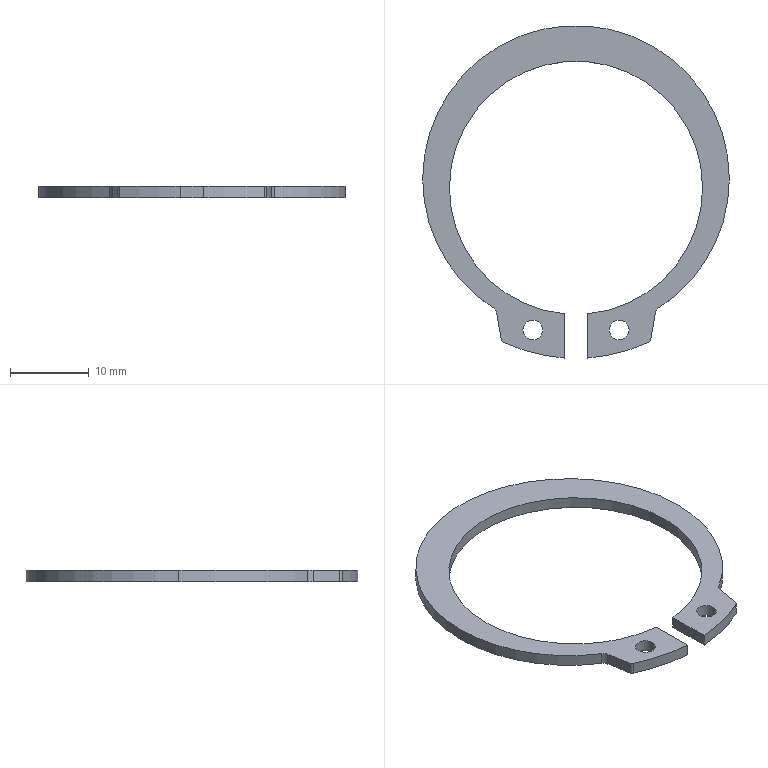Part | SolidWorks | features Extrusion 1 | 1 solid | 22 faces | box 39 x 42.278 x 1.5 mm | volume 631.207 mm3 | cylinder 16 | plane 6 | commonest cylinder face diameters 2.5 x4 32.2 x3 39 x3 1 x2 2 x2 43.4 x2
STEP:
#1=CARTESIAN_POINT('',(4.25,-19.212,0.75));
#2=VERTEX_POINT('',#1);
#3=CARTESIAN_POINT('',(6.75,-19.212,0.75));
#4=VERTEX_POINT('',#3);
#5=CARTESIAN_POINT('',(5.5,-19.212,0.75));
#6=DIRECTION('',(0.,0.,1.));
#7=DIRECTION('',(-1.,0.,0.));
#8=AXIS2_PLACEMENT_3D('',#5,#6,#7);
#9=CIRCLE('',#8,1.25);
#10=EDGE_CURVE('',#2,#4,#9,.T.);
#11=ORIENTED_EDGE('',*,*,#10,.T.);
#12=CARTESIAN_POINT('',(6.75,-19.212,-0.75));
#13=VERTEX_POINT('',#12);
#14=CARTESIAN_POINT('',(6.75,-19.212,0.75));
#15=DIRECTION('',(0.,0.,-1.));
#16=VECTOR('',#15,1000.);
#17=LINE('',#14,#16);
#18=EDGE_CURVE('',#4,#13,#17,.T.);
#19=ORIENTED_EDGE('',*,*,#18,.T.);
#20=CARTESIAN_POINT('',(4.25,-19.212,-0.75));
#21=VERTEX_POINT('',#20);
#22=CARTESIAN_POINT('',(5.5,-19.212,-0.75));
#23=DIRECTION('',(0.,0.,1.));
#24=DIRECTION('',(-1.,0.,0.));
#25=AXIS2_PLACEMENT_3D('',#22,#23,#24);
#26=CIRCLE('',#25,1.25);
#27=EDGE_CURVE('',#21,#13,#26,.T.);
#28=ORIENTED_EDGE('',*,*,#27,.F.);
#29=CARTESIAN_POINT('',(4.25,-19.212,0.75));
#30=DIRECTION('',(0.,0.,-1.));
#31=VECTOR('',#30,1000.);
#32=LINE('',#29,#31);
#33=EDGE_CURVE('',#2,#21,#32,.T.);
#34=ORIENTED_EDGE('',*,*,#33,.F.);
#35=EDGE_LOOP('',(#11,#19,#28,#34));
#36=FACE_OUTER_BOUND('',#35,.T.);
#37=CARTESIAN_POINT('',(5.5,-19.212,0.75));
#38=DIRECTION('',(0.,0.,-1.));
#39=DIRECTION('',(-1.,0.,0.));
#40=AXIS2_PLACEMENT_3D('',#37,#38,#39);
#41=CYLINDRICAL_SURFACE('',#40,1.25);
#42=ADVANCED_FACE('',(#36),#41,.F.);
#43=CARTESIAN_POINT('',(-6.75,-19.212,0.75));
#44=VERTEX_POINT('',#43);
#45=CARTESIAN_POINT('',(-4.25,-19.212,0.75));
#46=VERTEX_POINT('',#45);
#47=CARTESIAN_POINT('',(-5.5,-19.212,0.75));
#48=DIRECTION('',(0.,0.,1.));
#49=DIRECTION('',(1.,0.,0.));
#50=AXIS2_PLACEMENT_3D('',#47,#48,#49);
#51=CIRCLE('',#50,1.25);
#52=EDGE_CURVE('',#44,#46,#51,.T.);
#53=ORIENTED_EDGE('',*,*,#52,.T.);
#54=CARTESIAN_POINT('',(-4.25,-19.212,-0.75));
#55=VERTEX_POINT('',#54);
#56=CARTESIAN_POINT('',(-4.25,-19.212,0.75));
#57=DIRECTION('',(0.,0.,-1.));
#58=VECTOR('',#57,1000.);
#59=LINE('',#56,#58);
#60=EDGE_CURVE('',#46,#55,#59,.T.);
#61=ORIENTED_EDGE('',*,*,#60,.T.);
#62=CARTESIAN_POINT('',(-6.75,-19.212,-0.75));
#63=VERTEX_POINT('',#62);
#64=CARTESIAN_POINT('',(-5.5,-19.212,-0.75));
#65=DIRECTION('',(0.,0.,1.));
#66=DIRECTION('',(1.,0.,0.));
#67=AXIS2_PLACEMENT_3D('',#64,#65,#66);
#68=CIRCLE('',#67,1.25);
#69=EDGE_CURVE('',#63,#55,#68,.T.);
#70=ORIENTED_EDGE('',*,*,#69,.F.);
#71=CARTESIAN_POINT('',(-6.75,-19.212,0.75));
#72=DIRECTION('',(0.,0.,-1.));
#73=VECTOR('',#72,1000.);
#74=LINE('',#71,#73);
#75=EDGE_CURVE('',#44,#63,#74,.T.);
#76=ORIENTED_EDGE('',*,*,#75,.F.);
#77=EDGE_LOOP('',(#53,#61,#70,#76));
#78=FACE_OUTER_BOUND('',#77,.T.);
#79=CARTESIAN_POINT('',(-5.5,-19.212,0.75));
#80=DIRECTION('',(0.,0.,-1.));
#81=DIRECTION('',(-1.,0.,0.));
#82=AXIS2_PLACEMENT_3D('',#79,#80,#81);
#83=CYLINDRICAL_SURFACE('',#82,1.25);
#84=ADVANCED_FACE('',(#78),#83,.F.);
#85=CARTESIAN_POINT('',(19.5,0.,0.75));
#86=VERTEX_POINT('',#85);
#87=CARTESIAN_POINT('',(-19.5,0.,0.75));
#88=VERTEX_POINT('',#87);
#89=CARTESIAN_POINT('',(0.,0.,0.75));
#90=DIRECTION('',(0.,0.,1.));
#91=DIRECTION('',(1.,0.,0.));
#92=AXIS2_PLACEMENT_3D('',#89,#90,#91);
#93=CIRCLE('',#92,19.5);
#94=EDGE_CURVE('',#86,#88,#93,.T.);
#95=ORIENTED_EDGE('',*,*,#94,.F.);
#96=CARTESIAN_POINT('',(19.5,0.,-0.75));
#97=VERTEX_POINT('',#96);
#98=CARTESIAN_POINT('',(19.5,0.,0.75));
#99=DIRECTION('',(0.,0.,-1.));
#100=VECTOR('',#99,1000.);
#101=LINE('',#98,#100);
#102=EDGE_CURVE('',#86,#97,#101,.T.);
#103=ORIENTED_EDGE('',*,*,#102,.T.);
#104=CARTESIAN_POINT('',(-19.5,0.,-0.75));
#105=VERTEX_POINT('',#104);
#106=CARTESIAN_POINT('',(0.,0.,-0.75));
#107=DIRECTION('',(0.,0.,1.));
#108=DIRECTION('',(1.,0.,0.));
#109=AXIS2_PLACEMENT_3D('',#106,#107,#108);
#110=CIRCLE('',#109,19.5);
#111=EDGE_CURVE('',#97,#105,#110,.T.);
#112=ORIENTED_EDGE('',*,*,#111,.T.);
#113=CARTESIAN_POINT('',(-19.5,0.,0.75));
#114=DIRECTION('',(0.,0.,-1.));
#115=VECTOR('',#114,1000.);
#116=LINE('',#113,#115);
#117=EDGE_CURVE('',#88,#105,#116,.T.);
#118=ORIENTED_EDGE('',*,*,#117,.F.);
#119=EDGE_LOOP('',(#95,#103,#112,#118));
#120=FACE_OUTER_BOUND('',#119,.T.);
#121=CARTESIAN_POINT('',(0.,0.,0.75));
#122=DIRECTION('',(0.,0.,-1.));
#123=DIRECTION('',(-1.,0.,0.));
#124=AXIS2_PLACEMENT_3D('',#121,#122,#123);
#125=CYLINDRICAL_SURFACE('',#124,19.5);
#126=ADVANCED_FACE('',(#120),#125,.T.);
#127=CARTESIAN_POINT('',(-10.532,-16.411,0.75));
#128=VERTEX_POINT('',#127);
#129=CARTESIAN_POINT('',(0.,0.,0.75));
#130=DIRECTION('',(0.,0.,1.));
#131=DIRECTION('',(1.,0.,0.));
#132=AXIS2_PLACEMENT_3D('',#129,#130,#131);
#133=CIRCLE('',#132,19.5);
#134=EDGE_CURVE('',#88,#128,#133,.T.);
#135=ORIENTED_EDGE('',*,*,#134,.F.);
#136=ORIENTED_EDGE('',*,*,#117,.T.);
#137=CARTESIAN_POINT('',(-10.532,-16.411,-0.75));
#138=VERTEX_POINT('',#137);
#139=CARTESIAN_POINT('',(0.,0.,-0.75));
#140=DIRECTION('',(0.,0.,1.));
#141=DIRECTION('',(1.,0.,0.));
#142=AXIS2_PLACEMENT_3D('',#139,#140,#141);
#143=CIRCLE('',#142,19.5);
#144=EDGE_CURVE('',#105,#138,#143,.T.);
#145=ORIENTED_EDGE('',*,*,#144,.T.);
#146=CARTESIAN_POINT('',(-10.532,-16.411,0.75));
#147=DIRECTION('',(0.,0.,-1.));
#148=VECTOR('',#147,1000.);
#149=LINE('',#146,#148);
#150=EDGE_CURVE('',#128,#138,#149,.T.);
#151=ORIENTED_EDGE('',*,*,#150,.F.);
#152=EDGE_LOOP('',(#135,#136,#145,#151));
#153=FACE_OUTER_BOUND('',#152,.T.);
#154=CARTESIAN_POINT('',(0.,0.,0.75));
#155=DIRECTION('',(0.,0.,-1.));
#156=DIRECTION('',(-1.,0.,0.));
#157=AXIS2_PLACEMENT_3D('',#154,#155,#156);
#158=CYLINDRICAL_SURFACE('',#157,19.5);
#159=ADVANCED_FACE('',(#153),#158,.T.);
#160=CARTESIAN_POINT('',(16.1,-1.13,0.75));
#161=VERTEX_POINT('',#160);
#162=CARTESIAN_POINT('',(1.5,-17.16,0.75));
#163=VERTEX_POINT('',#162);
#164=CARTESIAN_POINT('',(0.,-1.13,0.75));
#165=DIRECTION('',(0.,0.,-1.));
#166=DIRECTION('',(1.,0.,0.));
#167=AXIS2_PLACEMENT_3D('',#164,#165,#166);
#168=CIRCLE('',#167,16.1);
#169=EDGE_CURVE('',#161,#163,#168,.T.);
#170=ORIENTED_EDGE('',*,*,#169,.F.);
#171=CARTESIAN_POINT('',(16.1,-1.13,-0.75));
#172=VERTEX_POINT('',#171);
#173=CARTESIAN_POINT('',(16.1,-1.13,0.75));
#174=DIRECTION('',(0.,0.,-1.));
#175=VECTOR('',#174,1000.);
#176=LINE('',#173,#175);
#177=EDGE_CURVE('',#161,#172,#176,.T.);
#178=ORIENTED_EDGE('',*,*,#177,.T.);
#179=CARTESIAN_POINT('',(1.5,-17.16,-0.75));
#180=VERTEX_POINT('',#179);
#181=CARTESIAN_POINT('',(0.,-1.13,-0.75));
#182=DIRECTION('',(0.,0.,-1.));
#183=DIRECTION('',(1.,0.,0.));
#184=AXIS2_PLACEMENT_3D('',#181,#182,#183);
#185=CIRCLE('',#184,16.1);
#186=EDGE_CURVE('',#172,#180,#185,.T.);
#187=ORIENTED_EDGE('',*,*,#186,.T.);
#188=CARTESIAN_POINT('',(1.5,-17.16,0.75));
#189=DIRECTION('',(0.,0.,-1.));
#190=VECTOR('',#189,1000.);
#191=LINE('',#188,#190);
#192=EDGE_CURVE('',#163,#180,#191,.T.);
#193=ORIENTED_EDGE('',*,*,#192,.F.);
#194=EDGE_LOOP('',(#170,#178,#187,#193));
#195=FACE_OUTER_BOUND('',#194,.T.);
#196=CARTESIAN_POINT('',(0.,-1.13,0.75));
#197=DIRECTION('',(0.,0.,-1.));
#198=DIRECTION('',(-1.,0.,0.));
#199=AXIS2_PLACEMENT_3D('',#196,#197,#198);
#200=CYLINDRICAL_SURFACE('',#199,16.1);
#201=ADVANCED_FACE('',(#195),#200,.F.);
#202=ORIENTED_EDGE('',*,*,#177,.F.);
#203=CARTESIAN_POINT('',(-16.1,-1.13,0.75));
#204=VERTEX_POINT('',#203);
#205=CARTESIAN_POINT('',(0.,-1.13,0.75));
#206=DIRECTION('',(0.,0.,-1.));
#207=DIRECTION('',(1.,0.,0.));
#208=AXIS2_PLACEMENT_3D('',#205,#206,#207);
#209=CIRCLE('',#208,16.1);
#210=EDGE_CURVE('',#204,#161,#209,.T.);
#211=ORIENTED_EDGE('',*,*,#210,.F.);
#212=CARTESIAN_POINT('',(-16.1,-1.13,-0.75));
#213=VERTEX_POINT('',#212);
#214=CARTESIAN_POINT('',(-16.1,-1.13,0.75));
#215=DIRECTION('',(0.,0.,-1.));
#216=VECTOR('',#215,1000.);
#217=LINE('',#214,#216);
#218=EDGE_CURVE('',#204,#213,#217,.T.);
#219=ORIENTED_EDGE('',*,*,#218,.T.);
#220=CARTESIAN_POINT('',(0.,-1.13,-0.75));
#221=DIRECTION('',(0.,0.,-1.));
#222=DIRECTION('',(1.,0.,0.));
#223=AXIS2_PLACEMENT_3D('',#220,#221,#222);
#224=CIRCLE('',#223,16.1);
#225=EDGE_CURVE('',#213,#172,#224,.T.);
#226=ORIENTED_EDGE('',*,*,#225,.T.);
#227=EDGE_LOOP('',(#202,#211,#219,#226));
#228=FACE_OUTER_BOUND('',#227,.T.);
#229=CARTESIAN_POINT('',(0.,-1.13,0.75));
#230=DIRECTION('',(0.,0.,-1.));
#231=DIRECTION('',(-1.,0.,0.));
#232=AXIS2_PLACEMENT_3D('',#229,#230,#231);
#233=CYLINDRICAL_SURFACE('',#232,16.1);
#234=ADVANCED_FACE('',(#228),#233,.F.);
#235=ORIENTED_EDGE('',*,*,#52,.F.);
#236=CARTESIAN_POINT('',(-5.5,-19.212,0.75));
#237=DIRECTION('',(0.,0.,1.));
#238=DIRECTION('',(1.,0.,0.));
#239=AXIS2_PLACEMENT_3D('',#236,#237,#238);
#240=CIRCLE('',#239,1.25);
#241=EDGE_CURVE('',#46,#44,#240,.T.);
#242=ORIENTED_EDGE('',*,*,#241,.F.);
#243=EDGE_LOOP('',(#235,#242));
#244=FACE_BOUND('',#243,.T.);
#245=CARTESIAN_POINT('',(-10.087,-17.079,0.75));
#246=VERTEX_POINT('',#245);
#247=CARTESIAN_POINT('',(-11.072,-17.253,0.75));
#248=DIRECTION('',(0.,0.,-1.));
#249=DIRECTION('',(1.,0.,0.));
#250=AXIS2_PLACEMENT_3D('',#247,#248,#249);
#251=CIRCLE('',#250,1.);
#252=EDGE_CURVE('',#128,#246,#251,.T.);
#253=ORIENTED_EDGE('',*,*,#252,.T.);
#254=CARTESIAN_POINT('',(-9.5,-20.408,0.75));
#255=VERTEX_POINT('',#254);
#256=CARTESIAN_POINT('',(-10.087,-17.079,0.75));
#257=DIRECTION('',(0.1736,-0.9848,0.));
#258=VECTOR('',#257,1000.);
#259=LINE('',#256,#258);
#260=EDGE_CURVE('',#246,#255,#259,.T.);
#261=ORIENTED_EDGE('',*,*,#260,.T.);
#262=CARTESIAN_POINT('',(-9.22,-20.774,0.75));
#263=VERTEX_POINT('',#262);
#264=CARTESIAN_POINT('',(-9.008,-20.321,0.75));
#265=DIRECTION('',(0.,0.,1.));
#266=DIRECTION('',(-1.,0.,0.));
#267=AXIS2_PLACEMENT_3D('',#264,#265,#266);
#268=CIRCLE('',#267,0.5);
#269=EDGE_CURVE('',#255,#263,#268,.T.);
#270=ORIENTED_EDGE('',*,*,#269,.T.);
#271=CARTESIAN_POINT('',(-1.5,-22.778,0.75));
#272=VERTEX_POINT('',#271);
#273=CARTESIAN_POINT('',(0.,-1.13,0.75));
#274=DIRECTION('',(0.,0.,1.));
#275=DIRECTION('',(-1.,0.,0.));
#276=AXIS2_PLACEMENT_3D('',#273,#274,#275);
#277=CIRCLE('',#276,21.7);
#278=EDGE_CURVE('',#263,#272,#277,.T.);
#279=ORIENTED_EDGE('',*,*,#278,.T.);
#280=CARTESIAN_POINT('',(-1.5,-17.16,0.75));
#281=VERTEX_POINT('',#280);
#282=CARTESIAN_POINT('',(-1.5,-17.16,0.75));
#283=DIRECTION('',(0.,1.,0.));
#284=VECTOR('',#283,1000.);
#285=LINE('',#282,#284);
#286=EDGE_CURVE('',#272,#281,#285,.T.);
#287=ORIENTED_EDGE('',*,*,#286,.T.);
#288=CARTESIAN_POINT('',(0.,-1.13,0.75));
#289=DIRECTION('',(0.,0.,-1.));
#290=DIRECTION('',(1.,0.,0.));
#291=AXIS2_PLACEMENT_3D('',#288,#289,#290);
#292=CIRCLE('',#291,16.1);
#293=EDGE_CURVE('',#281,#204,#292,.T.);
#294=ORIENTED_EDGE('',*,*,#293,.T.);
#295=ORIENTED_EDGE('',*,*,#210,.T.);
#296=ORIENTED_EDGE('',*,*,#169,.T.);
#297=CARTESIAN_POINT('',(1.5,-22.778,0.75));
#298=VERTEX_POINT('',#297);
#299=CARTESIAN_POINT('',(1.5,-17.16,0.75));
#300=DIRECTION('',(0.,-1.,0.));
#301=VECTOR('',#300,1000.);
#302=LINE('',#299,#301);
#303=EDGE_CURVE('',#163,#298,#302,.T.);
#304=ORIENTED_EDGE('',*,*,#303,.T.);
#305=CARTESIAN_POINT('',(9.22,-20.774,0.75));
#306=VERTEX_POINT('',#305);
#307=CARTESIAN_POINT('',(0.,-1.13,0.75));
#308=DIRECTION('',(0.,0.,1.));
#309=DIRECTION('',(1.,0.,0.));
#310=AXIS2_PLACEMENT_3D('',#307,#308,#309);
#311=CIRCLE('',#310,21.7);
#312=EDGE_CURVE('',#298,#306,#311,.T.);
#313=ORIENTED_EDGE('',*,*,#312,.T.);
#314=CARTESIAN_POINT('',(9.5,-20.408,0.75));
#315=VERTEX_POINT('',#314);
#316=CARTESIAN_POINT('',(9.008,-20.321,0.75));
#317=DIRECTION('',(0.,0.,1.));
#318=DIRECTION('',(1.,0.,0.));
#319=AXIS2_PLACEMENT_3D('',#316,#317,#318);
#320=CIRCLE('',#319,0.5);
#321=EDGE_CURVE('',#306,#315,#320,.T.);
#322=ORIENTED_EDGE('',*,*,#321,.T.);
#323=CARTESIAN_POINT('',(10.087,-17.079,0.75));
#324=VERTEX_POINT('',#323);
#325=CARTESIAN_POINT('',(10.087,-17.079,0.75));
#326=DIRECTION('',(0.1736,0.9848,0.));
#327=VECTOR('',#326,1000.);
#328=LINE('',#325,#327);
#329=EDGE_CURVE('',#315,#324,#328,.T.);
#330=ORIENTED_EDGE('',*,*,#329,.T.);
#331=CARTESIAN_POINT('',(10.532,-16.411,0.75));
#332=VERTEX_POINT('',#331);
#333=CARTESIAN_POINT('',(11.072,-17.253,0.75));
#334=DIRECTION('',(0.,0.,-1.));
#335=DIRECTION('',(-1.,0.,0.));
#336=AXIS2_PLACEMENT_3D('',#333,#334,#335);
#337=CIRCLE('',#336,1.);
#338=EDGE_CURVE('',#324,#332,#337,.T.);
#339=ORIENTED_EDGE('',*,*,#338,.T.);
#340=CARTESIAN_POINT('',(0.,0.,0.75));
#341=DIRECTION('',(0.,0.,1.));
#342=DIRECTION('',(1.,0.,0.));
#343=AXIS2_PLACEMENT_3D('',#340,#341,#342);
#344=CIRCLE('',#343,19.5);
#345=EDGE_CURVE('',#332,#86,#344,.T.);
#346=ORIENTED_EDGE('',*,*,#345,.T.);
#347=ORIENTED_EDGE('',*,*,#94,.T.);
#348=ORIENTED_EDGE('',*,*,#134,.T.);
#349=EDGE_LOOP('',(#253,#261,#270,#279,#287,#294,#295,#296,#304,#313,#322,#330,#339,#346,#347,#348));
#350=FACE_OUTER_BOUND('',#349,.T.);
#351=ORIENTED_EDGE('',*,*,#10,.F.);
#352=CARTESIAN_POINT('',(5.5,-19.212,0.75));
#353=DIRECTION('',(0.,0.,1.));
#354=DIRECTION('',(-1.,0.,0.));
#355=AXIS2_PLACEMENT_3D('',#352,#353,#354);
#356=CIRCLE('',#355,1.25);
#357=EDGE_CURVE('',#4,#2,#356,.T.);
#358=ORIENTED_EDGE('',*,*,#357,.F.);
#359=EDGE_LOOP('',(#351,#358));
#360=FACE_BOUND('',#359,.T.);
#361=CARTESIAN_POINT('',(-11.072,-17.253,0.75));
#362=DIRECTION('',(0.,0.,1.));
#363=DIRECTION('',(1.,0.,0.));
#364=AXIS2_PLACEMENT_3D('',#361,#362,#363);
#365=PLANE('',#364);
#366=ADVANCED_FACE('',(#244,#350,#360),#365,.T.);
#367=ORIENTED_EDGE('',*,*,#150,.T.);
#368=CARTESIAN_POINT('',(-10.087,-17.079,-0.75));
#369=VERTEX_POINT('',#368);
#370=CARTESIAN_POINT('',(-11.072,-17.253,-0.75));
#371=DIRECTION('',(0.,0.,-1.));
#372=DIRECTION('',(1.,0.,0.));
#373=AXIS2_PLACEMENT_3D('',#370,#371,#372);
#374=CIRCLE('',#373,1.);
#375=EDGE_CURVE('',#138,#369,#374,.T.);
#376=ORIENTED_EDGE('',*,*,#375,.T.);
#377=CARTESIAN_POINT('',(-10.087,-17.079,0.75));
#378=DIRECTION('',(0.,0.,-1.));
#379=VECTOR('',#378,1000.);
#380=LINE('',#377,#379);
#381=EDGE_CURVE('',#246,#369,#380,.T.);
#382=ORIENTED_EDGE('',*,*,#381,.F.);
#383=ORIENTED_EDGE('',*,*,#252,.F.);
#384=EDGE_LOOP('',(#367,#376,#382,#383));
#385=FACE_OUTER_BOUND('',#384,.T.);
#386=CARTESIAN_POINT('',(-11.072,-17.253,0.75));
#387=DIRECTION('',(0.,0.,-1.));
#388=DIRECTION('',(-1.,0.,0.));
#389=AXIS2_PLACEMENT_3D('',#386,#387,#388);
#390=CYLINDRICAL_SURFACE('',#389,1.);
#391=ADVANCED_FACE('',(#385),#390,.F.);
#392=ORIENTED_EDGE('',*,*,#381,.T.);
#393=CARTESIAN_POINT('',(-9.5,-20.408,-0.75));
#394=VERTEX_POINT('',#393);
#395=CARTESIAN_POINT('',(-10.087,-17.079,-0.75));
#396=DIRECTION('',(0.1736,-0.9848,0.));
#397=VECTOR('',#396,1000.);
#398=LINE('',#395,#397);
#399=EDGE_CURVE('',#369,#394,#398,.T.);
#400=ORIENTED_EDGE('',*,*,#399,.T.);
#401=CARTESIAN_POINT('',(-9.5,-20.408,0.75));
#402=DIRECTION('',(0.,0.,-1.));
#403=VECTOR('',#402,1000.);
#404=LINE('',#401,#403);
#405=EDGE_CURVE('',#255,#394,#404,.T.);
#406=ORIENTED_EDGE('',*,*,#405,.F.);
#407=ORIENTED_EDGE('',*,*,#260,.F.);
#408=EDGE_LOOP('',(#392,#400,#406,#407));
#409=FACE_OUTER_BOUND('',#408,.T.);
#410=CARTESIAN_POINT('',(-10.087,-17.079,0.75));
#411=DIRECTION('',(0.9848,0.1736,0.));
#412=DIRECTION('',(-0.1736,0.9848,0.));
#413=AXIS2_PLACEMENT_3D('',#410,#411,#412);
#414=PLANE('',#413);
#415=ADVANCED_FACE('',(#409),#414,.F.);
#416=ORIENTED_EDGE('',*,*,#405,.T.);
#417=CARTESIAN_POINT('',(-9.22,-20.774,-0.75));
#418=VERTEX_POINT('',#417);
#419=CARTESIAN_POINT('',(-9.008,-20.321,-0.75));
#420=DIRECTION('',(0.,0.,1.));
#421=DIRECTION('',(-1.,0.,0.));
#422=AXIS2_PLACEMENT_3D('',#419,#420,#421);
#423=CIRCLE('',#422,0.5);
#424=EDGE_CURVE('',#394,#418,#423,.T.);
#425=ORIENTED_EDGE('',*,*,#424,.T.);
#426=CARTESIAN_POINT('',(-9.22,-20.774,0.75));
#427=DIRECTION('',(0.,0.,-1.));
#428=VECTOR('',#427,1000.);
#429=LINE('',#426,#428);
#430=EDGE_CURVE('',#263,#418,#429,.T.);
#431=ORIENTED_EDGE('',*,*,#430,.F.);
#432=ORIENTED_EDGE('',*,*,#269,.F.);
#433=EDGE_LOOP('',(#416,#425,#431,#432));
#434=FACE_OUTER_BOUND('',#433,.T.);
#435=CARTESIAN_POINT('',(-9.008,-20.321,0.75));
#436=DIRECTION('',(0.,0.,-1.));
#437=DIRECTION('',(-1.,0.,0.));
#438=AXIS2_PLACEMENT_3D('',#435,#436,#437);
#439=CYLINDRICAL_SURFACE('',#438,0.5);
#440=ADVANCED_FACE('',(#434),#439,.T.);
#441=ORIENTED_EDGE('',*,*,#430,.T.);
#442=CARTESIAN_POINT('',(-1.5,-22.778,-0.75));
#443=VERTEX_POINT('',#442);
#444=CARTESIAN_POINT('',(0.,-1.13,-0.75));
#445=DIRECTION('',(0.,0.,1.));
#446=DIRECTION('',(-1.,0.,0.));
#447=AXIS2_PLACEMENT_3D('',#444,#445,#446);
#448=CIRCLE('',#447,21.7);
#449=EDGE_CURVE('',#418,#443,#448,.T.);
#450=ORIENTED_EDGE('',*,*,#449,.T.);
#451=CARTESIAN_POINT('',(-1.5,-22.778,0.75));
#452=DIRECTION('',(0.,0.,-1.));
#453=VECTOR('',#452,1000.);
#454=LINE('',#451,#453);
#455=EDGE_CURVE('',#272,#443,#454,.T.);
#456=ORIENTED_EDGE('',*,*,#455,.F.);
#457=ORIENTED_EDGE('',*,*,#278,.F.);
#458=EDGE_LOOP('',(#441,#450,#456,#457));
#459=FACE_OUTER_BOUND('',#458,.T.);
#460=CARTESIAN_POINT('',(0.,-1.13,0.75));
#461=DIRECTION('',(0.,0.,-1.));
#462=DIRECTION('',(-1.,0.,0.));
#463=AXIS2_PLACEMENT_3D('',#460,#461,#462);
#464=CYLINDRICAL_SURFACE('',#463,21.7);
#465=ADVANCED_FACE('',(#459),#464,.T.);
#466=ORIENTED_EDGE('',*,*,#455,.T.);
#467=CARTESIAN_POINT('',(-1.5,-17.16,-0.75));
#468=VERTEX_POINT('',#467);
#469=CARTESIAN_POINT('',(-1.5,-17.16,-0.75));
#470=DIRECTION('',(0.,1.,0.));
#471=VECTOR('',#470,1000.);
#472=LINE('',#469,#471);
#473=EDGE_CURVE('',#443,#468,#472,.T.);
#474=ORIENTED_EDGE('',*,*,#473,.T.);
#475=CARTESIAN_POINT('',(-1.5,-17.16,0.75));
#476=DIRECTION('',(0.,0.,-1.));
#477=VECTOR('',#476,1000.);
#478=LINE('',#475,#477);
#479=EDGE_CURVE('',#281,#468,#478,.T.);
#480=ORIENTED_EDGE('',*,*,#479,.F.);
#481=ORIENTED_EDGE('',*,*,#286,.F.);
#482=EDGE_LOOP('',(#466,#474,#480,#481));
#483=FACE_OUTER_BOUND('',#482,.T.);
#484=CARTESIAN_POINT('',(-1.5,-17.16,0.75));
#485=DIRECTION('',(-1.,0.,0.));
#486=DIRECTION('',(0.,-1.,0.));
#487=AXIS2_PLACEMENT_3D('',#484,#485,#486);
#488=PLANE('',#487);
#489=ADVANCED_FACE('',(#483),#488,.F.);
#490=ORIENTED_EDGE('',*,*,#218,.F.);
#491=ORIENTED_EDGE('',*,*,#293,.F.);
#492=ORIENTED_EDGE('',*,*,#479,.T.);
#493=CARTESIAN_POINT('',(0.,-1.13,-0.75));
#494=DIRECTION('',(0.,0.,-1.));
#495=DIRECTION('',(1.,0.,0.));
#496=AXIS2_PLACEMENT_3D('',#493,#494,#495);
#497=CIRCLE('',#496,16.1);
#498=EDGE_CURVE('',#468,#213,#497,.T.);
#499=ORIENTED_EDGE('',*,*,#498,.T.);
#500=EDGE_LOOP('',(#490,#491,#492,#499));
#501=FACE_OUTER_BOUND('',#500,.T.);
#502=CARTESIAN_POINT('',(0.,-1.13,0.75));
#503=DIRECTION('',(0.,0.,-1.));
#504=DIRECTION('',(-1.,0.,0.));
#505=AXIS2_PLACEMENT_3D('',#502,#503,#504);
#506=CYLINDRICAL_SURFACE('',#505,16.1);
#507=ADVANCED_FACE('',(#501),#506,.F.);
#508=ORIENTED_EDGE('',*,*,#192,.T.);
#509=CARTESIAN_POINT('',(1.5,-22.778,-0.75));
#510=VERTEX_POINT('',#509);
#511=CARTESIAN_POINT('',(1.5,-17.16,-0.75));
#512=DIRECTION('',(0.,-1.,0.));
#513=VECTOR('',#512,1000.);
#514=LINE('',#511,#513);
#515=EDGE_CURVE('',#180,#510,#514,.T.);
#516=ORIENTED_EDGE('',*,*,#515,.T.);
#517=CARTESIAN_POINT('',(1.5,-22.778,0.75));
#518=DIRECTION('',(0.,0.,-1.));
#519=VECTOR('',#518,1000.);
#520=LINE('',#517,#519);
#521=EDGE_CURVE('',#298,#510,#520,.T.);
#522=ORIENTED_EDGE('',*,*,#521,.F.);
#523=ORIENTED_EDGE('',*,*,#303,.F.);
#524=EDGE_LOOP('',(#508,#516,#522,#523));
#525=FACE_OUTER_BOUND('',#524,.T.);
#526=CARTESIAN_POINT('',(1.5,-17.16,0.75));
#527=DIRECTION('',(1.,0.,0.));
#528=DIRECTION('',(0.,1.,0.));
#529=AXIS2_PLACEMENT_3D('',#526,#527,#528);
#530=PLANE('',#529);
#531=ADVANCED_FACE('',(#525),#530,.F.);
#532=ORIENTED_EDGE('',*,*,#521,.T.);
#533=CARTESIAN_POINT('',(9.22,-20.774,-0.75));
#534=VERTEX_POINT('',#533);
#535=CARTESIAN_POINT('',(0.,-1.13,-0.75));
#536=DIRECTION('',(0.,0.,1.));
#537=DIRECTION('',(1.,0.,0.));
#538=AXIS2_PLACEMENT_3D('',#535,#536,#537);
#539=CIRCLE('',#538,21.7);
#540=EDGE_CURVE('',#510,#534,#539,.T.);
#541=ORIENTED_EDGE('',*,*,#540,.T.);
#542=CARTESIAN_POINT('',(9.22,-20.774,0.75));
#543=DIRECTION('',(0.,0.,-1.));
#544=VECTOR('',#543,1000.);
#545=LINE('',#542,#544);
#546=EDGE_CURVE('',#306,#534,#545,.T.);
#547=ORIENTED_EDGE('',*,*,#546,.F.);
#548=ORIENTED_EDGE('',*,*,#312,.F.);
#549=EDGE_LOOP('',(#532,#541,#547,#548));
#550=FACE_OUTER_BOUND('',#549,.T.);
#551=CARTESIAN_POINT('',(0.,-1.13,0.75));
#552=DIRECTION('',(0.,0.,-1.));
#553=DIRECTION('',(-1.,0.,0.));
#554=AXIS2_PLACEMENT_3D('',#551,#552,#553);
#555=CYLINDRICAL_SURFACE('',#554,21.7);
#556=ADVANCED_FACE('',(#550),#555,.T.);
#557=ORIENTED_EDGE('',*,*,#546,.T.);
#558=CARTESIAN_POINT('',(9.5,-20.408,-0.75));
#559=VERTEX_POINT('',#558);
#560=CARTESIAN_POINT('',(9.008,-20.321,-0.75));
#561=DIRECTION('',(0.,0.,1.));
#562=DIRECTION('',(1.,0.,0.));
#563=AXIS2_PLACEMENT_3D('',#560,#561,#562);
#564=CIRCLE('',#563,0.5);
#565=EDGE_CURVE('',#534,#559,#564,.T.);
#566=ORIENTED_EDGE('',*,*,#565,.T.);
#567=CARTESIAN_POINT('',(9.5,-20.408,0.75));
#568=DIRECTION('',(0.,0.,-1.));
#569=VECTOR('',#568,1000.);
#570=LINE('',#567,#569);
#571=EDGE_CURVE('',#315,#559,#570,.T.);
#572=ORIENTED_EDGE('',*,*,#571,.F.);
#573=ORIENTED_EDGE('',*,*,#321,.F.);
#574=EDGE_LOOP('',(#557,#566,#572,#573));
#575=FACE_OUTER_BOUND('',#574,.T.);
#576=CARTESIAN_POINT('',(9.008,-20.321,0.75));
#577=DIRECTION('',(0.,0.,-1.));
#578=DIRECTION('',(-1.,0.,0.));
#579=AXIS2_PLACEMENT_3D('',#576,#577,#578);
#580=CYLINDRICAL_SURFACE('',#579,0.5);
#581=ADVANCED_FACE('',(#575),#580,.T.);
#582=ORIENTED_EDGE('',*,*,#571,.T.);
#583=CARTESIAN_POINT('',(10.087,-17.079,-0.75));
#584=VERTEX_POINT('',#583);
#585=CARTESIAN_POINT('',(10.087,-17.079,-0.75));
#586=DIRECTION('',(0.1736,0.9848,0.));
#587=VECTOR('',#586,1000.);
#588=LINE('',#585,#587);
#589=EDGE_CURVE('',#559,#584,#588,.T.);
#590=ORIENTED_EDGE('',*,*,#589,.T.);
#591=CARTESIAN_POINT('',(10.087,-17.079,0.75));
#592=DIRECTION('',(0.,0.,-1.));
#593=VECTOR('',#592,1000.);
#594=LINE('',#591,#593);
#595=EDGE_CURVE('',#324,#584,#594,.T.);
#596=ORIENTED_EDGE('',*,*,#595,.F.);
#597=ORIENTED_EDGE('',*,*,#329,.F.);
#598=EDGE_LOOP('',(#582,#590,#596,#597));
#599=FACE_OUTER_BOUND('',#598,.T.);
#600=CARTESIAN_POINT('',(10.087,-17.079,0.75));
#601=DIRECTION('',(-0.9848,0.1736,0.));
#602=DIRECTION('',(-0.1736,-0.9848,0.));
#603=AXIS2_PLACEMENT_3D('',#600,#601,#602);
#604=PLANE('',#603);
#605=ADVANCED_FACE('',(#599),#604,.F.);
#606=ORIENTED_EDGE('',*,*,#595,.T.);
#607=CARTESIAN_POINT('',(10.532,-16.411,-0.75));
#608=VERTEX_POINT('',#607);
#609=CARTESIAN_POINT('',(11.072,-17.253,-0.75));
#610=DIRECTION('',(0.,0.,-1.));
#611=DIRECTION('',(-1.,0.,0.));
#612=AXIS2_PLACEMENT_3D('',#609,#610,#611);
#613=CIRCLE('',#612,1.);
#614=EDGE_CURVE('',#584,#608,#613,.T.);
#615=ORIENTED_EDGE('',*,*,#614,.T.);
#616=CARTESIAN_POINT('',(10.532,-16.411,0.75));
#617=DIRECTION('',(0.,0.,-1.));
#618=VECTOR('',#617,1000.);
#619=LINE('',#616,#618);
#620=EDGE_CURVE('',#332,#608,#619,.T.);
#621=ORIENTED_EDGE('',*,*,#620,.F.);
#622=ORIENTED_EDGE('',*,*,#338,.F.);
#623=EDGE_LOOP('',(#606,#615,#621,#622));
#624=FACE_OUTER_BOUND('',#623,.T.);
#625=CARTESIAN_POINT('',(11.072,-17.253,0.75));
#626=DIRECTION('',(0.,0.,-1.));
#627=DIRECTION('',(-1.,0.,0.));
#628=AXIS2_PLACEMENT_3D('',#625,#626,#627);
#629=CYLINDRICAL_SURFACE('',#628,1.);
#630=ADVANCED_FACE('',(#624),#629,.F.);
#631=ORIENTED_EDGE('',*,*,#102,.F.);
#632=ORIENTED_EDGE('',*,*,#345,.F.);
#633=ORIENTED_EDGE('',*,*,#620,.T.);
#634=CARTESIAN_POINT('',(0.,0.,-0.75));
#635=DIRECTION('',(0.,0.,1.));
#636=DIRECTION('',(1.,0.,0.));
#637=AXIS2_PLACEMENT_3D('',#634,#635,#636);
#638=CIRCLE('',#637,19.5);
#639=EDGE_CURVE('',#608,#97,#638,.T.);
#640=ORIENTED_EDGE('',*,*,#639,.T.);
#641=EDGE_LOOP('',(#631,#632,#633,#640));
#642=FACE_OUTER_BOUND('',#641,.T.);
#643=CARTESIAN_POINT('',(0.,0.,0.75));
#644=DIRECTION('',(0.,0.,-1.));
#645=DIRECTION('',(-1.,0.,0.));
#646=AXIS2_PLACEMENT_3D('',#643,#644,#645);
#647=CYLINDRICAL_SURFACE('',#646,19.5);
#648=ADVANCED_FACE('',(#642),#647,.T.);
#649=ORIENTED_EDGE('',*,*,#60,.F.);
#650=ORIENTED_EDGE('',*,*,#241,.T.);
#651=ORIENTED_EDGE('',*,*,#75,.T.);
#652=CARTESIAN_POINT('',(-5.5,-19.212,-0.75));
#653=DIRECTION('',(0.,0.,1.));
#654=DIRECTION('',(1.,0.,0.));
#655=AXIS2_PLACEMENT_3D('',#652,#653,#654);
#656=CIRCLE('',#655,1.25);
#657=EDGE_CURVE('',#55,#63,#656,.T.);
#658=ORIENTED_EDGE('',*,*,#657,.F.);
#659=EDGE_LOOP('',(#649,#650,#651,#658));
#660=FACE_OUTER_BOUND('',#659,.T.);
#661=CARTESIAN_POINT('',(-5.5,-19.212,0.75));
#662=DIRECTION('',(0.,0.,-1.));
#663=DIRECTION('',(-1.,0.,0.));
#664=AXIS2_PLACEMENT_3D('',#661,#662,#663);
#665=CYLINDRICAL_SURFACE('',#664,1.25);
#666=ADVANCED_FACE('',(#660),#665,.F.);
#667=ORIENTED_EDGE('',*,*,#18,.F.);
#668=ORIENTED_EDGE('',*,*,#357,.T.);
#669=ORIENTED_EDGE('',*,*,#33,.T.);
#670=CARTESIAN_POINT('',(5.5,-19.212,-0.75));
#671=DIRECTION('',(0.,0.,1.));
#672=DIRECTION('',(-1.,0.,0.));
#673=AXIS2_PLACEMENT_3D('',#670,#671,#672);
#674=CIRCLE('',#673,1.25);
#675=EDGE_CURVE('',#13,#21,#674,.T.);
#676=ORIENTED_EDGE('',*,*,#675,.F.);
#677=EDGE_LOOP('',(#667,#668,#669,#676));
#678=FACE_OUTER_BOUND('',#677,.T.);
#679=CARTESIAN_POINT('',(5.5,-19.212,0.75));
#680=DIRECTION('',(0.,0.,-1.));
#681=DIRECTION('',(-1.,0.,0.));
#682=AXIS2_PLACEMENT_3D('',#679,#680,#681);
#683=CYLINDRICAL_SURFACE('',#682,1.25);
#684=ADVANCED_FACE('',(#678),#683,.F.);
#685=ORIENTED_EDGE('',*,*,#27,.T.);
#686=ORIENTED_EDGE('',*,*,#675,.T.);
#687=EDGE_LOOP('',(#685,#686));
#688=FACE_BOUND('',#687,.T.);
#689=ORIENTED_EDGE('',*,*,#69,.T.);
#690=ORIENTED_EDGE('',*,*,#657,.T.);
#691=EDGE_LOOP('',(#689,#690));
#692=FACE_BOUND('',#691,.T.);
#693=ORIENTED_EDGE('',*,*,#375,.F.);
#694=ORIENTED_EDGE('',*,*,#144,.F.);
#695=ORIENTED_EDGE('',*,*,#111,.F.);
#696=ORIENTED_EDGE('',*,*,#639,.F.);
#697=ORIENTED_EDGE('',*,*,#614,.F.);
#698=ORIENTED_EDGE('',*,*,#589,.F.);
#699=ORIENTED_EDGE('',*,*,#565,.F.);
#700=ORIENTED_EDGE('',*,*,#540,.F.);
#701=ORIENTED_EDGE('',*,*,#515,.F.);
#702=ORIENTED_EDGE('',*,*,#186,.F.);
#703=ORIENTED_EDGE('',*,*,#225,.F.);
#704=ORIENTED_EDGE('',*,*,#498,.F.);
#705=ORIENTED_EDGE('',*,*,#473,.F.);
#706=ORIENTED_EDGE('',*,*,#449,.F.);
#707=ORIENTED_EDGE('',*,*,#424,.F.);
#708=ORIENTED_EDGE('',*,*,#399,.F.);
#709=EDGE_LOOP('',(#693,#694,#695,#696,#697,#698,#699,#700,#701,#702,#703,#704,#705,#706,#707,#708));
#710=FACE_OUTER_BOUND('',#709,.T.);
#711=CARTESIAN_POINT('',(-11.072,-17.253,-0.75));
#712=DIRECTION('',(0.,0.,1.));
#713=DIRECTION('',(1.,0.,0.));
#714=AXIS2_PLACEMENT_3D('',#711,#712,#713);
#715=PLANE('',#714);
#716=ADVANCED_FACE('',(#688,#692,#710),#715,.F.);
#717=CLOSED_SHELL('',(#42,#84,#126,#159,#201,#234,#366,#391,#415,#440,#465,#489,#507,#531,#556,#581,#605,#630,#648,#666,#684,#716));
#718=MANIFOLD_SOLID_BREP('',#717);
#719=CARTESIAN_POINT('',(0.,0.,0.));
#720=DIRECTION('',(0.,0.,1.));
#721=DIRECTION('',(1.,0.,0.));
#722=AXIS2_PLACEMENT_3D('',#719,#720,#721);
#723=(LENGTH_UNIT()NAMED_UNIT(*)SI_UNIT(.MILLI.,.METRE.));
#724=UNCERTAINTY_MEASURE_WITH_UNIT(LENGTH_MEASURE(0.00001),#723,'','');
#725=(NAMED_UNIT(*)PLANE_ANGLE_UNIT()SI_UNIT($,.RADIAN.));
#726=(NAMED_UNIT(*)SI_UNIT($,.STERADIAN.)SOLID_ANGLE_UNIT());
#727=(GEOMETRIC_REPRESENTATION_CONTEXT(3)GLOBAL_UNCERTAINTY_ASSIGNED_CONTEXT((#724))GLOBAL_UNIT_ASSIGNED_CONTEXT((#723,#725,#726))REPRESENTATION_CONTEXT('',''));
#728=ADVANCED_BREP_SHAPE_REPRESENTATION('',(#718,#722),#727);